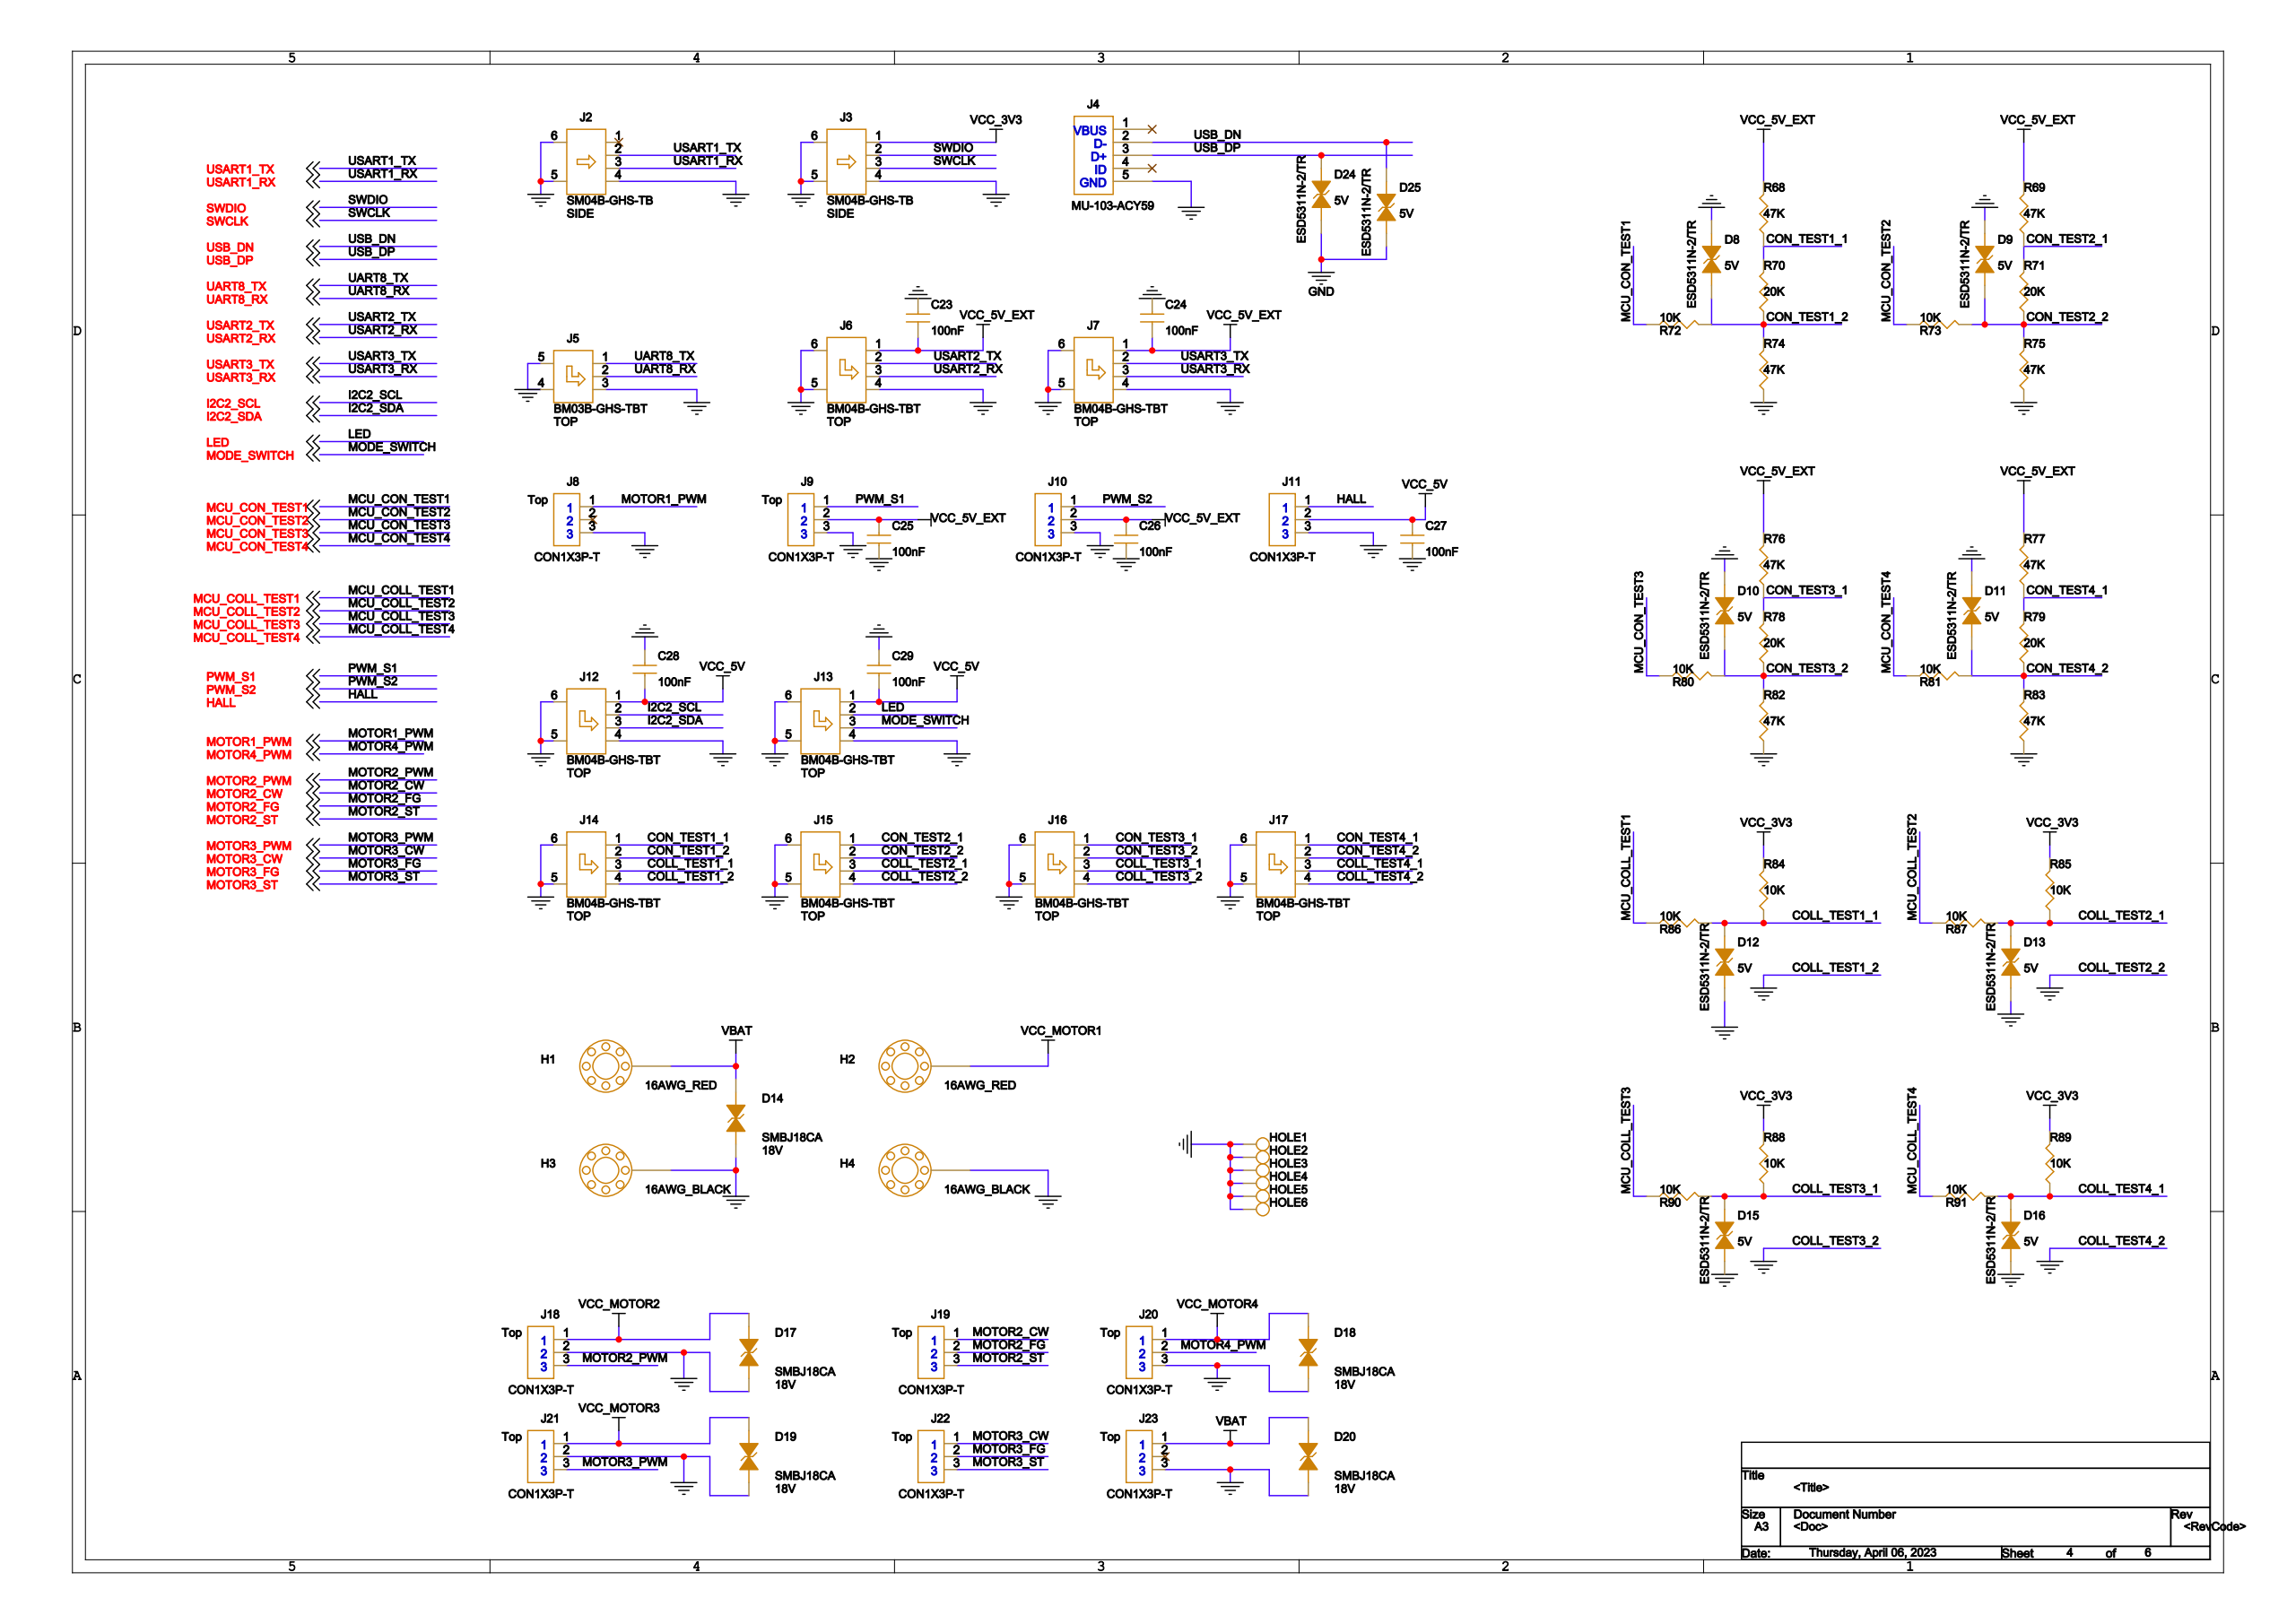Circuit board | Cadence Allegro | 278 parts | 154 nets | one sheet of the schematic
Parts on this sheet (reference | value | footprint):
C23 | 100nF | C0402
C24 | 100nF | C0402
C25 | 100nF | C0402
C26 | 100nF | C0402
C27 | 100nF | C0402
C28 | 100nF | C0402
C29 | 100nF | C0402
D8 | ESD5311N-2/TR | DFN1006-2L
D9 | ESD5311N-2/TR | DFN1006-2L
D10 | ESD5311N-2/TR | DFN1006-2L
D11 | ESD5311N-2/TR | DFN1006-2L
D12 | ESD5311N-2/TR | DFN1006-2L
D13 | ESD5311N-2/TR | DFN1006-2L
D14 | SMBJ18CA | SMBJ18CA
D15 | ESD5311N-2/TR | DFN1006-2L
D16 | ESD5311N-2/TR | DFN1006-2L
D17 | SMBJ18CA | SMBJ18CA
D18 | SMBJ18CA | SMBJ18CA
D19 | SMBJ18CA | SMBJ18CA
D20 | SMBJ18CA | SMBJ18CA
D24 | ESD5311N-2/TR | DFN1006-2L
D25 | ESD5311N-2/TR | DFN1006-2L
H1 | 16AWG_RED | HOLE_3P8D2P4_P
H2 | 16AWG_RED | HOLE_3P8D2P4_P
H3 | 16AWG_BLACK | HOLE_3P8D2P4_P
H4 | 16AWG_BLACK | HOLE_3P8D2P4_P
HOLE1 | T POINT R | HOLE_5P4D2P5_P
HOLE2 | T POINT R | HOLE_5P4D2P5_P
HOLE3 | T POINT R | HOLE_5P4D2P5_P
HOLE4 | T POINT R | HOLE_5P4D2P5_P
HOLE5 | T POINT R | HOLE_5P4D2P5_P
HOLE6 | T POINT R | HOLE_5P4D2P5_P
J2 | SM04B-GHS-TB | SM04B-GHS-TB
J3 | SM04B-GHS-TB | SM04B-GHS-TB
J4 | MU-103-ACY59 | SMD
J5 | BM03B-GHS-TBT | BM03B-GHS-TBT
J6 | BM04B-GHS-TBT | BM04B-GHS-TBT
J7 | BM04B-GHS-TBT | BM04B-GHS-TBT
J8 | CON1X3P-T | CON1X3P-T
J9 | CON1X3P-T | CON1X3P-T
J10 | CON1X3P-T | CON1X3P-T
J11 | CON1X3P-T | CON1X3P-T
J12 | BM04B-GHS-TBT | BM04B-GHS-TBT
J13 | BM04B-GHS-TBT | BM04B-GHS-TBT
J14 | BM04B-GHS-TBT | BM04B-GHS-TBT
J15 | BM04B-GHS-TBT | BM04B-GHS-TBT
J16 | BM04B-GHS-TBT | BM04B-GHS-TBT
J17 | BM04B-GHS-TBT | BM04B-GHS-TBT
J18 | CON1X3P-T | CON1X3P-T
J19 | CON1X3P-T | CON1X3P-T
J20 | CON1X3P-T | CON1X3P-T
J21 | CON1X3P-T | CON1X3P-T
J22 | CON1X3P-T | CON1X3P-T
J23 | CON1X3P-T | CON1X3P-T
R68 | 47K | R0402
R69 | 47K | R0402
R70 | 20K | R0402
R71 | 20K | R0402
R72 | 10K | R0402
R73 | 10K | R0402
R74 | 47K | R0402
R75 | 47K | R0402
R76 | 47K | R0402
R77 | 47K | R0402
R78 | 20K | R0402
R79 | 20K | R0402
R80 | 10K | R0402
R81 | 10K | R0402
R82 | 47K | R0402
R83 | 47K | R0402
R84 | 10K | R0402
R85 | 10K | R0402
R86 | 10K | R0402
R87 | 10K | R0402
R88 | 10K | R0402
R89 | 10K | R0402
R90 | 10K | R0402
R91 | 10K | R0402
Nets of these parts (net: part-pin ...):
GND: C23-2 C24-2 C25-1 C26-1 C27-1 C28-2 C29-2 D8-1 D9-1 D10-1 D11-1 D12-2 D13-2 D14-2 D15-2 D16-2 D17-2 D18-2 D19-2 D20-2 D24-2 D25-2 H3-1 H4-1 HOLE1-1 HOLE2-1 HOLE3-1 HOLE4-1 HOLE5-1 HOLE6-1 J2-4 J2-5 J2-6 J3-4 J3-5 J3-6 J4-5 J5-3 J5-4 J5-5 J6-4 J6-5 J6-6 J7-4 J7-5 J7-6 J8-3 J9-3 J10-3 J11-3 J12-4 J12-5 J12-6 J13-4 J13-5 J13-6 J14-4 J14-5 J14-6 J15-4 J15-5 J15-6 J16-4 J16-5 J16-6 J17-4 J17-5 J17-6 J18-2 J20-3 J21-2 J23-3 R74-1 R75-1 R82-1 R83-1
CON_TEST3_2: D10-2 J16-2 R78-1 R80-2 R82-2
CON_TEST4_2: D11-2 J17-2 R79-1 R81-2 R83-2
COLL_TEST1_1: D12-1 J14-3 R84-1 R86-2
COLL_TEST2_1: D13-1 J15-3 R85-1 R87-2
COLL_TEST3_1: D15-1 J16-3 R88-1 R90-2
COLL_TEST4_1: D16-1 J17-3 R89-1 R91-2
USB_DP: D24-1 J4-3
USB_DN: D25-1 J4-2
CON_TEST1_2: D8-2 J14-2 R70-1 R72-2 R74-2
CON_TEST2_2: D9-2 J15-2 R71-1 R73-2 R75-2
VCC_3V3: J3-1 R84-2 R85-2 R88-2 R89-2
VCC_5V_EXT: C23-1 C24-1 C25-2 C26-2 J6-1 J7-1 J9-2 J10-2 R68-2 R69-2 R76-2 R77-2
VCC_5V: C27-2 C28-1 C29-1 J11-2 J12-1 J13-1
VBAT: D14-1 D20-1 H1-1 J23-1
VCC_MOTOR2: D17-1 J18-1
VCC_MOTOR4: D18-1 J20-1
VCC_MOTOR3: D19-1 J21-1
VCC_MOTOR1: H2-1
PWM_S2: J10-1
HALL: J11-1
MOTOR2_PWM: J18-3
MOTOR2_CW: J19-1
MOTOR2_FG: J19-2
MOTOR2_ST: J19-3
MOTOR4_PWM: J20-2
MOTOR3_PWM: J21-3
MOTOR3_CW: J22-1
MOTOR3_FG: J22-2
MOTOR3_ST: J22-3
MOTOR1_PWM: J8-1
PWM_S1: J9-1
I2C2_SCL: J12-2
I2C2_SDA: J12-3
LED: J13-2
MODE_SWITCH: J13-3
CON_TEST1_1: J14-1 R68-1 R70-2
CON_TEST2_1: J15-1 R69-1 R71-2
CON_TEST3_1: J16-1 R76-1 R78-2
CON_TEST4_1: J17-1 R77-1 R79-2
USART2_TX: J6-2
USART2_RX: J6-3
USART3_TX: J7-2
USART3_RX: J7-3
USART1_TX: J2-2
USART1_RX: J2-3
SWDIO: J3-2
SWCLK: J3-3
UART8_TX: J5-1
UART8_RX: J5-2
MCU_CON_TEST1: R72-1
MCU_CON_TEST2: R73-1
MCU_CON_TEST3: R80-1
MCU_CON_TEST4: R81-1
MCU_COLL_TEST1: R86-1
MCU_COLL_TEST2: R87-1
MCU_COLL_TEST3: R90-1
MCU_COLL_TEST4: R91-1